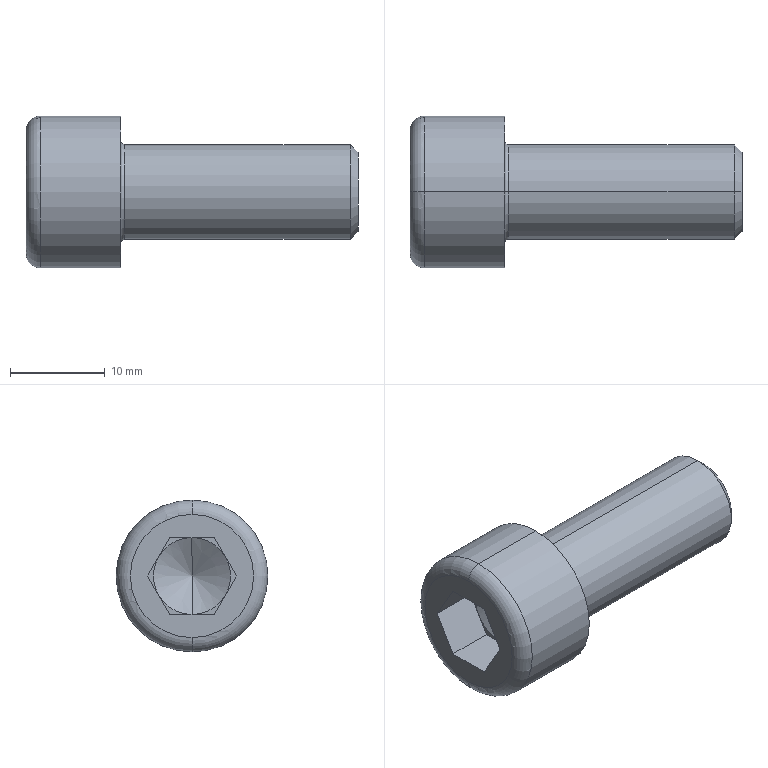Part | STEP file | socket head cap screw_iso_ISO 4762 M10 x 25 --- 25N | 1 solid | 27 faces | box 35 x 16 x 16 mm | volume 3616 mm3 | plane 15 | cone 4 | torus 4 | cylinder 4 | commonest cylinder face diameters 10 x2 16 x2